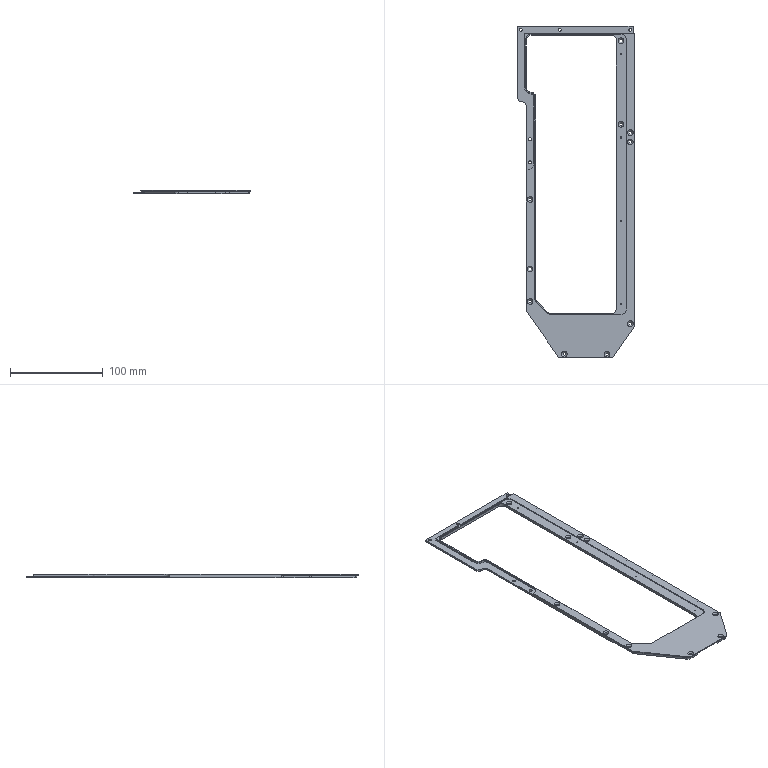Part | 1 solid | 127 faces | box 127 x 358 x 4 mm | volume 42050 mm3 | cylinder 68 | plane 39 | cone 20 | commonest cylinder face diameters 3.2 x28 10 x16 1.6 x8 12 x6 4 x4 3 x2